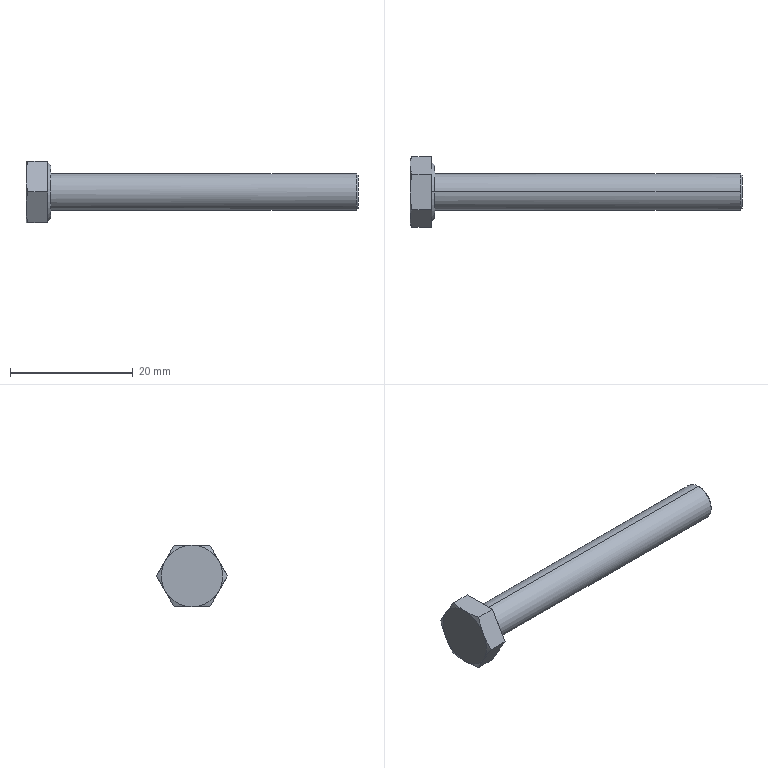Part | STEP file | hex head bolts-full thread grade c gb_GB_FASTENER_BOLT_HHBFTC M6X50-S | 1 solid | 22 faces | box 54 x 11.547 x 10 mm | volume 1749 mm3 | cone 10 | plane 10 | cylinder 2 | commonest cylinder face diameters 6 x2
STEP:
#1=CARTESIAN_POINT('',(53.7,3.,0.));
#2=VERTEX_POINT('',#1);
#3=CARTESIAN_POINT('',(53.7,0.,-3.));
#4=VERTEX_POINT('',#3);
#5=CARTESIAN_POINT('',(53.7,0.,0.));
#6=DIRECTION('',(-1.,0.,0.));
#7=DIRECTION('',(0.,0.,1.));
#8=AXIS2_PLACEMENT_3D('',#5,#6,#7);
#9=CIRCLE('',#8,3.);
#10=EDGE_CURVE('',#2,#4,#9,.T.);
#11=ORIENTED_EDGE('',*,*,#10,.T.);
#12=CARTESIAN_POINT('',(4.,0.,-3.));
#13=VERTEX_POINT('',#12);
#14=CARTESIAN_POINT('',(54.,0.,-3.));
#15=DIRECTION('',(-1.,0.,0.));
#16=VECTOR('',#15,1000.);
#17=LINE('',#14,#16);
#18=EDGE_CURVE('',#4,#13,#17,.T.);
#19=ORIENTED_EDGE('',*,*,#18,.T.);
#20=CARTESIAN_POINT('',(4.,0.,3.));
#21=VERTEX_POINT('',#20);
#22=CARTESIAN_POINT('',(4.,0.,0.));
#23=DIRECTION('',(1.,0.,0.));
#24=DIRECTION('',(0.,0.,1.));
#25=AXIS2_PLACEMENT_3D('',#22,#23,#24);
#26=CIRCLE('',#25,3.);
#27=EDGE_CURVE('',#13,#21,#26,.T.);
#28=ORIENTED_EDGE('',*,*,#27,.T.);
#29=CARTESIAN_POINT('',(53.7,0.,3.));
#30=VERTEX_POINT('',#29);
#31=CARTESIAN_POINT('',(54.,0.,3.));
#32=DIRECTION('',(-1.,0.,0.));
#33=VECTOR('',#32,1000.);
#34=LINE('',#31,#33);
#35=EDGE_CURVE('',#30,#21,#34,.T.);
#36=ORIENTED_EDGE('',*,*,#35,.F.);
#37=CARTESIAN_POINT('',(53.7,0.,0.));
#38=DIRECTION('',(-1.,0.,0.));
#39=DIRECTION('',(0.,0.,1.));
#40=AXIS2_PLACEMENT_3D('',#37,#38,#39);
#41=CIRCLE('',#40,3.);
#42=EDGE_CURVE('',#30,#2,#41,.T.);
#43=ORIENTED_EDGE('',*,*,#42,.T.);
#44=EDGE_LOOP('',(#11,#19,#28,#36,#43));
#45=FACE_OUTER_BOUND('',#44,.T.);
#46=CARTESIAN_POINT('',(54.,0.,0.));
#47=DIRECTION('',(-1.,0.,0.));
#48=DIRECTION('',(0.,0.,1.));
#49=AXIS2_PLACEMENT_3D('',#46,#47,#48);
#50=CYLINDRICAL_SURFACE('',#49,3.);
#51=ADVANCED_FACE('',(#45),#50,.T.);
#52=CARTESIAN_POINT('',(54.,-2.7,0.));
#53=VERTEX_POINT('',#52);
#54=CARTESIAN_POINT('',(54.,2.7,0.));
#55=VERTEX_POINT('',#54);
#56=CARTESIAN_POINT('',(54.,0.,0.));
#57=DIRECTION('',(-1.,0.,0.));
#58=DIRECTION('',(0.,-1.,0.));
#59=AXIS2_PLACEMENT_3D('',#56,#57,#58);
#60=CIRCLE('',#59,2.7);
#61=EDGE_CURVE('',#53,#55,#60,.T.);
#62=ORIENTED_EDGE('',*,*,#61,.T.);
#63=CARTESIAN_POINT('',(53.7,3.,0.));
#64=DIRECTION('',(-0.7071,0.7071,0.));
#65=VECTOR('',#64,1000.);
#66=LINE('',#63,#65);
#67=EDGE_CURVE('',#55,#2,#66,.T.);
#68=ORIENTED_EDGE('',*,*,#67,.T.);
#69=ORIENTED_EDGE('',*,*,#42,.F.);
#70=CARTESIAN_POINT('',(53.7,-3.,0.));
#71=VERTEX_POINT('',#70);
#72=CARTESIAN_POINT('',(53.7,0.,0.));
#73=DIRECTION('',(-1.,0.,0.));
#74=DIRECTION('',(0.,0.,1.));
#75=AXIS2_PLACEMENT_3D('',#72,#73,#74);
#76=CIRCLE('',#75,3.);
#77=EDGE_CURVE('',#71,#30,#76,.T.);
#78=ORIENTED_EDGE('',*,*,#77,.F.);
#79=CARTESIAN_POINT('',(53.7,-3.,0.));
#80=DIRECTION('',(-0.7071,-0.7071,0.));
#81=VECTOR('',#80,1000.);
#82=LINE('',#79,#81);
#83=EDGE_CURVE('',#53,#71,#82,.T.);
#84=ORIENTED_EDGE('',*,*,#83,.F.);
#85=EDGE_LOOP('',(#62,#68,#69,#78,#84));
#86=FACE_OUTER_BOUND('',#85,.T.);
#87=CARTESIAN_POINT('',(53.7,0.,0.));
#88=DIRECTION('',(-1.,0.,0.));
#89=DIRECTION('',(0.,-1.,0.));
#90=AXIS2_PLACEMENT_3D('',#87,#88,#89);
#91=CONICAL_SURFACE('',#90,3.,0.7854);
#92=ADVANCED_FACE('',(#86),#91,.T.);
#93=CARTESIAN_POINT('',(4.,0.,4.37));
#94=VERTEX_POINT('',#93);
#95=CARTESIAN_POINT('',(4.,0.,-4.37));
#96=VERTEX_POINT('',#95);
#97=CARTESIAN_POINT('',(4.,0.,0.));
#98=DIRECTION('',(-1.,0.,0.));
#99=DIRECTION('',(0.,0.,1.));
#100=AXIS2_PLACEMENT_3D('',#97,#98,#99);
#101=CIRCLE('',#100,4.37);
#102=EDGE_CURVE('',#94,#96,#101,.T.);
#103=ORIENTED_EDGE('',*,*,#102,.T.);
#104=CARTESIAN_POINT('',(3.5,0.,-4.87));
#105=VERTEX_POINT('',#104);
#106=CARTESIAN_POINT('',(3.5,0.,-4.87));
#107=DIRECTION('',(-0.7071,0.,-0.7071));
#108=VECTOR('',#107,1000.);
#109=LINE('',#106,#108);
#110=EDGE_CURVE('',#96,#105,#109,.T.);
#111=ORIENTED_EDGE('',*,*,#110,.T.);
#112=CARTESIAN_POINT('',(3.5,0.,4.87));
#113=VERTEX_POINT('',#112);
#114=CARTESIAN_POINT('',(3.5,0.,0.));
#115=DIRECTION('',(1.,0.,0.));
#116=DIRECTION('',(0.,0.,1.));
#117=AXIS2_PLACEMENT_3D('',#114,#115,#116);
#118=CIRCLE('',#117,4.87);
#119=EDGE_CURVE('',#105,#113,#118,.T.);
#120=ORIENTED_EDGE('',*,*,#119,.T.);
#121=CARTESIAN_POINT('',(3.5,0.,4.87));
#122=DIRECTION('',(-0.7071,0.,0.7071));
#123=VECTOR('',#122,1000.);
#124=LINE('',#121,#123);
#125=EDGE_CURVE('',#94,#113,#124,.T.);
#126=ORIENTED_EDGE('',*,*,#125,.F.);
#127=EDGE_LOOP('',(#103,#111,#120,#126));
#128=FACE_OUTER_BOUND('',#127,.T.);
#129=CARTESIAN_POINT('',(3.5,0.,0.));
#130=DIRECTION('',(-1.,0.,0.));
#131=DIRECTION('',(0.,0.,1.));
#132=AXIS2_PLACEMENT_3D('',#129,#130,#131);
#133=CONICAL_SURFACE('',#132,4.87,0.7854);
#134=ADVANCED_FACE('',(#128),#133,.T.);
#135=ORIENTED_EDGE('',*,*,#18,.F.);
#136=CARTESIAN_POINT('',(53.7,0.,0.));
#137=DIRECTION('',(-1.,0.,0.));
#138=DIRECTION('',(0.,0.,1.));
#139=AXIS2_PLACEMENT_3D('',#136,#137,#138);
#140=CIRCLE('',#139,3.);
#141=EDGE_CURVE('',#4,#71,#140,.T.);
#142=ORIENTED_EDGE('',*,*,#141,.T.);
#143=ORIENTED_EDGE('',*,*,#77,.T.);
#144=ORIENTED_EDGE('',*,*,#35,.T.);
#145=CARTESIAN_POINT('',(4.,0.,0.));
#146=DIRECTION('',(1.,0.,0.));
#147=DIRECTION('',(0.,0.,1.));
#148=AXIS2_PLACEMENT_3D('',#145,#146,#147);
#149=CIRCLE('',#148,3.);
#150=EDGE_CURVE('',#21,#13,#149,.T.);
#151=ORIENTED_EDGE('',*,*,#150,.T.);
#152=EDGE_LOOP('',(#135,#142,#143,#144,#151));
#153=FACE_OUTER_BOUND('',#152,.T.);
#154=CARTESIAN_POINT('',(54.,0.,0.));
#155=DIRECTION('',(-1.,0.,0.));
#156=DIRECTION('',(0.,0.,1.));
#157=AXIS2_PLACEMENT_3D('',#154,#155,#156);
#158=CYLINDRICAL_SURFACE('',#157,3.);
#159=ADVANCED_FACE('',(#153),#158,.T.);
#160=ORIENTED_EDGE('',*,*,#150,.F.);
#161=ORIENTED_EDGE('',*,*,#27,.F.);
#162=EDGE_LOOP('',(#160,#161));
#163=FACE_BOUND('',#162,.T.);
#164=ORIENTED_EDGE('',*,*,#102,.F.);
#165=CARTESIAN_POINT('',(4.,0.,0.));
#166=DIRECTION('',(-1.,0.,0.));
#167=DIRECTION('',(0.,0.,1.));
#168=AXIS2_PLACEMENT_3D('',#165,#166,#167);
#169=CIRCLE('',#168,4.37);
#170=EDGE_CURVE('',#96,#94,#169,.T.);
#171=ORIENTED_EDGE('',*,*,#170,.F.);
#172=EDGE_LOOP('',(#164,#171));
#173=FACE_OUTER_BOUND('',#172,.T.);
#174=CARTESIAN_POINT('',(4.,0.,10.));
#175=DIRECTION('',(-1.,0.,0.));
#176=DIRECTION('',(0.,0.,1.));
#177=AXIS2_PLACEMENT_3D('',#174,#175,#176);
#178=PLANE('',#177);
#179=ADVANCED_FACE('',(#163,#173),#178,.F.);
#180=ORIENTED_EDGE('',*,*,#67,.F.);
#181=CARTESIAN_POINT('',(54.,0.,0.));
#182=DIRECTION('',(-1.,0.,0.));
#183=DIRECTION('',(0.,-1.,0.));
#184=AXIS2_PLACEMENT_3D('',#181,#182,#183);
#185=CIRCLE('',#184,2.7);
#186=EDGE_CURVE('',#55,#53,#185,.T.);
#187=ORIENTED_EDGE('',*,*,#186,.T.);
#188=ORIENTED_EDGE('',*,*,#83,.T.);
#189=ORIENTED_EDGE('',*,*,#141,.F.);
#190=ORIENTED_EDGE('',*,*,#10,.F.);
#191=EDGE_LOOP('',(#180,#187,#188,#189,#190));
#192=FACE_OUTER_BOUND('',#191,.T.);
#193=CARTESIAN_POINT('',(53.7,0.,0.));
#194=DIRECTION('',(-1.,0.,0.));
#195=DIRECTION('',(0.,-1.,0.));
#196=AXIS2_PLACEMENT_3D('',#193,#194,#195);
#197=CONICAL_SURFACE('',#196,3.,0.7854);
#198=ADVANCED_FACE('',(#192),#197,.T.);
#199=ORIENTED_EDGE('',*,*,#110,.F.);
#200=ORIENTED_EDGE('',*,*,#170,.T.);
#201=ORIENTED_EDGE('',*,*,#125,.T.);
#202=CARTESIAN_POINT('',(3.5,0.,0.));
#203=DIRECTION('',(1.,0.,0.));
#204=DIRECTION('',(0.,0.,1.));
#205=AXIS2_PLACEMENT_3D('',#202,#203,#204);
#206=CIRCLE('',#205,4.87);
#207=EDGE_CURVE('',#113,#105,#206,.T.);
#208=ORIENTED_EDGE('',*,*,#207,.T.);
#209=EDGE_LOOP('',(#199,#200,#201,#208));
#210=FACE_OUTER_BOUND('',#209,.T.);
#211=CARTESIAN_POINT('',(3.5,0.,0.));
#212=DIRECTION('',(-1.,0.,0.));
#213=DIRECTION('',(0.,0.,1.));
#214=AXIS2_PLACEMENT_3D('',#211,#212,#213);
#215=CONICAL_SURFACE('',#214,4.87,0.7854);
#216=ADVANCED_FACE('',(#210),#215,.T.);
#217=ORIENTED_EDGE('',*,*,#61,.F.);
#218=ORIENTED_EDGE('',*,*,#186,.F.);
#219=EDGE_LOOP('',(#217,#218));
#220=FACE_OUTER_BOUND('',#219,.T.);
#221=CARTESIAN_POINT('',(54.,0.,0.));
#222=DIRECTION('',(1.,0.,0.));
#223=DIRECTION('',(0.,0.,-1.));
#224=AXIS2_PLACEMENT_3D('',#221,#222,#223);
#225=PLANE('',#224);
#226=ADVANCED_FACE('',(#220),#225,.T.);
#227=CARTESIAN_POINT('',(3.5,5.774,0.));
#228=VERTEX_POINT('',#227);
#229=CARTESIAN_POINT('',(3.5,2.887,5.));
#230=VERTEX_POINT('',#229);
#231=CARTESIAN_POINT('',(3.5,5.774,0.));
#232=DIRECTION('',(0.,-0.5,0.866));
#233=VECTOR('',#232,1000.);
#234=LINE('',#231,#233);
#235=EDGE_CURVE('',#228,#230,#234,.T.);
#236=ORIENTED_EDGE('',*,*,#235,.T.);
#237=CARTESIAN_POINT('',(3.5,-2.887,5.));
#238=VERTEX_POINT('',#237);
#239=CARTESIAN_POINT('',(3.5,4.87,5.));
#240=DIRECTION('',(0.,-1.,0.));
#241=VECTOR('',#240,1000.);
#242=LINE('',#239,#241);
#243=EDGE_CURVE('',#230,#238,#242,.T.);
#244=ORIENTED_EDGE('',*,*,#243,.T.);
#245=CARTESIAN_POINT('',(3.5,-5.774,0.));
#246=VERTEX_POINT('',#245);
#247=CARTESIAN_POINT('',(3.5,-2.887,5.));
#248=DIRECTION('',(0.,-0.5,-0.866));
#249=VECTOR('',#248,1000.);
#250=LINE('',#247,#249);
#251=EDGE_CURVE('',#238,#246,#250,.T.);
#252=ORIENTED_EDGE('',*,*,#251,.T.);
#253=CARTESIAN_POINT('',(3.5,-2.887,-5.));
#254=VERTEX_POINT('',#253);
#255=CARTESIAN_POINT('',(3.5,-5.774,0.));
#256=DIRECTION('',(0.,0.5,-0.866));
#257=VECTOR('',#256,1000.);
#258=LINE('',#255,#257);
#259=EDGE_CURVE('',#246,#254,#258,.T.);
#260=ORIENTED_EDGE('',*,*,#259,.T.);
#261=CARTESIAN_POINT('',(3.5,2.887,-5.));
#262=VERTEX_POINT('',#261);
#263=CARTESIAN_POINT('',(3.5,4.87,-5.));
#264=DIRECTION('',(0.,1.,0.));
#265=VECTOR('',#264,1000.);
#266=LINE('',#263,#265);
#267=EDGE_CURVE('',#254,#262,#266,.T.);
#268=ORIENTED_EDGE('',*,*,#267,.T.);
#269=CARTESIAN_POINT('',(3.5,2.887,-5.));
#270=DIRECTION('',(0.,0.5,0.866));
#271=VECTOR('',#270,1000.);
#272=LINE('',#269,#271);
#273=EDGE_CURVE('',#262,#228,#272,.T.);
#274=ORIENTED_EDGE('',*,*,#273,.T.);
#275=EDGE_LOOP('',(#236,#244,#252,#260,#268,#274));
#276=FACE_OUTER_BOUND('',#275,.T.);
#277=ORIENTED_EDGE('',*,*,#207,.F.);
#278=ORIENTED_EDGE('',*,*,#119,.F.);
#279=EDGE_LOOP('',(#277,#278));
#280=FACE_BOUND('',#279,.T.);
#281=CARTESIAN_POINT('',(3.5,4.87,0.));
#282=DIRECTION('',(1.,0.,0.));
#283=DIRECTION('',(0.,0.,-1.));
#284=AXIS2_PLACEMENT_3D('',#281,#282,#283);
#285=PLANE('',#284);
#286=ADVANCED_FACE('',(#276,#280),#285,.T.);
#287=CARTESIAN_POINT('',(0.2815,-2.887,5.));
#288=VERTEX_POINT('',#287);
#289=CARTESIAN_POINT('',(4.,-2.887,5.));
#290=DIRECTION('',(-1.,0.,0.));
#291=VECTOR('',#290,1000.);
#292=LINE('',#289,#291);
#293=EDGE_CURVE('',#238,#288,#292,.T.);
#294=ORIENTED_EDGE('',*,*,#293,.F.);
#295=ORIENTED_EDGE('',*,*,#243,.F.);
#296=CARTESIAN_POINT('',(0.2815,2.887,5.));
#297=VERTEX_POINT('',#296);
#298=CARTESIAN_POINT('',(4.,2.887,5.));
#299=DIRECTION('',(1.,0.,0.));
#300=VECTOR('',#299,1000.);
#301=LINE('',#298,#300);
#302=EDGE_CURVE('',#297,#230,#301,.T.);
#303=ORIENTED_EDGE('',*,*,#302,.F.);
#304=CARTESIAN_POINT('',(0.,0.,5.));
#305=VERTEX_POINT('',#304);
#306=CARTESIAN_POINT('',(0.,0.,5.));
#307=CARTESIAN_POINT('',(0.,0.9714,5.));
#308=CARTESIAN_POINT('',(0.1078,1.932,5.));
#309=CARTESIAN_POINT('',(0.2815,2.887,5.));
#310=B_SPLINE_CURVE_WITH_KNOTS('',3,(#306,#307,#308,#309),.UNSPECIFIED.,.F.,.F.,(4,4),(0.,0.0029),.UNSPECIFIED.);
#311=EDGE_CURVE('',#305,#297,#310,.T.);
#312=ORIENTED_EDGE('',*,*,#311,.F.);
#313=CARTESIAN_POINT('',(0.2815,-2.887,5.));
#314=CARTESIAN_POINT('',(0.1078,-1.932,5.));
#315=CARTESIAN_POINT('',(0.,-0.9714,5.));
#316=CARTESIAN_POINT('',(0.,0.,5.));
#317=B_SPLINE_CURVE_WITH_KNOTS('',3,(#313,#314,#315,#316),.UNSPECIFIED.,.F.,.F.,(4,4),(0.,0.0029),.UNSPECIFIED.);
#318=EDGE_CURVE('',#288,#305,#317,.T.);
#319=ORIENTED_EDGE('',*,*,#318,.F.);
#320=EDGE_LOOP('',(#294,#295,#303,#312,#319));
#321=FACE_OUTER_BOUND('',#320,.T.);
#322=CARTESIAN_POINT('',(4.,2.887,5.));
#323=DIRECTION('',(0.,0.,-1.));
#324=DIRECTION('',(0.,1.,0.));
#325=AXIS2_PLACEMENT_3D('',#322,#323,#324);
#326=PLANE('',#325);
#327=ADVANCED_FACE('',(#321),#326,.F.);
#328=ORIENTED_EDGE('',*,*,#302,.T.);
#329=ORIENTED_EDGE('',*,*,#235,.F.);
#330=CARTESIAN_POINT('',(0.2815,5.774,0.));
#331=VERTEX_POINT('',#330);
#332=CARTESIAN_POINT('',(4.,5.774,0.));
#333=DIRECTION('',(1.,0.,0.));
#334=VECTOR('',#333,1000.);
#335=LINE('',#332,#334);
#336=EDGE_CURVE('',#331,#228,#335,.T.);
#337=ORIENTED_EDGE('',*,*,#336,.F.);
#338=CARTESIAN_POINT('',(0.,4.33,2.5));
#339=VERTEX_POINT('',#338);
#340=CARTESIAN_POINT('',(0.,4.33,2.5));
#341=CARTESIAN_POINT('',(0.,4.816,1.659));
#342=CARTESIAN_POINT('',(0.1078,5.296,0.8266));
#343=CARTESIAN_POINT('',(0.2815,5.774,0.));
#344=B_SPLINE_CURVE_WITH_KNOTS('',3,(#340,#341,#342,#343),.UNSPECIFIED.,.F.,.F.,(4,4),(0.,0.0029),.UNSPECIFIED.);
#345=EDGE_CURVE('',#339,#331,#344,.T.);
#346=ORIENTED_EDGE('',*,*,#345,.F.);
#347=CARTESIAN_POINT('',(0.2815,2.887,5.));
#348=CARTESIAN_POINT('',(0.1078,3.364,4.173));
#349=CARTESIAN_POINT('',(0.,3.844,3.341));
#350=CARTESIAN_POINT('',(0.,4.33,2.5));
#351=B_SPLINE_CURVE_WITH_KNOTS('',3,(#347,#348,#349,#350),.UNSPECIFIED.,.F.,.F.,(4,4),(0.,0.0029),.UNSPECIFIED.);
#352=EDGE_CURVE('',#297,#339,#351,.T.);
#353=ORIENTED_EDGE('',*,*,#352,.F.);
#354=EDGE_LOOP('',(#328,#329,#337,#346,#353));
#355=FACE_OUTER_BOUND('',#354,.T.);
#356=CARTESIAN_POINT('',(4.,5.774,0.));
#357=DIRECTION('',(0.,-0.866,-0.5));
#358=DIRECTION('',(0.,0.5,-0.866));
#359=AXIS2_PLACEMENT_3D('',#356,#357,#358);
#360=PLANE('',#359);
#361=ADVANCED_FACE('',(#355),#360,.F.);
#362=ORIENTED_EDGE('',*,*,#336,.T.);
#363=ORIENTED_EDGE('',*,*,#273,.F.);
#364=CARTESIAN_POINT('',(0.2815,2.887,-5.));
#365=VERTEX_POINT('',#364);
#366=CARTESIAN_POINT('',(4.,2.887,-5.));
#367=DIRECTION('',(1.,0.,0.));
#368=VECTOR('',#367,1000.);
#369=LINE('',#366,#368);
#370=EDGE_CURVE('',#365,#262,#369,.T.);
#371=ORIENTED_EDGE('',*,*,#370,.F.);
#372=CARTESIAN_POINT('',(0.,4.33,-2.5));
#373=VERTEX_POINT('',#372);
#374=CARTESIAN_POINT('',(0.,4.33,-2.5));
#375=CARTESIAN_POINT('',(0.,3.844,-3.341));
#376=CARTESIAN_POINT('',(0.1078,3.364,-4.173));
#377=CARTESIAN_POINT('',(0.2815,2.887,-5.));
#378=B_SPLINE_CURVE_WITH_KNOTS('',3,(#374,#375,#376,#377),.UNSPECIFIED.,.F.,.F.,(4,4),(0.,0.0029),.UNSPECIFIED.);
#379=EDGE_CURVE('',#373,#365,#378,.T.);
#380=ORIENTED_EDGE('',*,*,#379,.F.);
#381=CARTESIAN_POINT('',(0.2815,5.774,0.));
#382=CARTESIAN_POINT('',(0.1078,5.296,-0.8266));
#383=CARTESIAN_POINT('',(0.,4.816,-1.659));
#384=CARTESIAN_POINT('',(0.,4.33,-2.5));
#385=B_SPLINE_CURVE_WITH_KNOTS('',3,(#381,#382,#383,#384),.UNSPECIFIED.,.F.,.F.,(4,4),(0.,0.0029),.UNSPECIFIED.);
#386=EDGE_CURVE('',#331,#373,#385,.T.);
#387=ORIENTED_EDGE('',*,*,#386,.F.);
#388=EDGE_LOOP('',(#362,#363,#371,#380,#387));
#389=FACE_OUTER_BOUND('',#388,.T.);
#390=CARTESIAN_POINT('',(4.,2.887,-5.));
#391=DIRECTION('',(0.,-0.866,0.5));
#392=DIRECTION('',(0.,-0.5,-0.866));
#393=AXIS2_PLACEMENT_3D('',#390,#391,#392);
#394=PLANE('',#393);
#395=ADVANCED_FACE('',(#389),#394,.F.);
#396=ORIENTED_EDGE('',*,*,#370,.T.);
#397=ORIENTED_EDGE('',*,*,#267,.F.);
#398=CARTESIAN_POINT('',(0.2815,-2.887,-5.));
#399=VERTEX_POINT('',#398);
#400=CARTESIAN_POINT('',(4.,-2.887,-5.));
#401=DIRECTION('',(1.,0.,0.));
#402=VECTOR('',#401,1000.);
#403=LINE('',#400,#402);
#404=EDGE_CURVE('',#399,#254,#403,.T.);
#405=ORIENTED_EDGE('',*,*,#404,.F.);
#406=CARTESIAN_POINT('',(0.,0.,-5.));
#407=VERTEX_POINT('',#406);
#408=CARTESIAN_POINT('',(0.,0.,-5.));
#409=CARTESIAN_POINT('',(0.,-0.9714,-5.));
#410=CARTESIAN_POINT('',(0.1078,-1.932,-5.));
#411=CARTESIAN_POINT('',(0.2815,-2.887,-5.));
#412=B_SPLINE_CURVE_WITH_KNOTS('',3,(#408,#409,#410,#411),.UNSPECIFIED.,.F.,.F.,(4,4),(0.,0.0029),.UNSPECIFIED.);
#413=EDGE_CURVE('',#407,#399,#412,.T.);
#414=ORIENTED_EDGE('',*,*,#413,.F.);
#415=CARTESIAN_POINT('',(0.2815,2.887,-5.));
#416=CARTESIAN_POINT('',(0.1078,1.932,-5.));
#417=CARTESIAN_POINT('',(0.,0.9714,-5.));
#418=CARTESIAN_POINT('',(0.,0.,-5.));
#419=B_SPLINE_CURVE_WITH_KNOTS('',3,(#415,#416,#417,#418),.UNSPECIFIED.,.F.,.F.,(4,4),(0.,0.0029),.UNSPECIFIED.);
#420=EDGE_CURVE('',#365,#407,#419,.T.);
#421=ORIENTED_EDGE('',*,*,#420,.F.);
#422=EDGE_LOOP('',(#396,#397,#405,#414,#421));
#423=FACE_OUTER_BOUND('',#422,.T.);
#424=CARTESIAN_POINT('',(4.,-2.887,-5.));
#425=DIRECTION('',(0.,0.,1.));
#426=DIRECTION('',(1.,0.,0.));
#427=AXIS2_PLACEMENT_3D('',#424,#425,#426);
#428=PLANE('',#427);
#429=ADVANCED_FACE('',(#423),#428,.F.);
#430=ORIENTED_EDGE('',*,*,#404,.T.);
#431=ORIENTED_EDGE('',*,*,#259,.F.);
#432=CARTESIAN_POINT('',(0.2815,-5.774,0.));
#433=VERTEX_POINT('',#432);
#434=CARTESIAN_POINT('',(4.,-5.774,0.));
#435=DIRECTION('',(1.,0.,0.));
#436=VECTOR('',#435,1000.);
#437=LINE('',#434,#436);
#438=EDGE_CURVE('',#433,#246,#437,.T.);
#439=ORIENTED_EDGE('',*,*,#438,.F.);
#440=CARTESIAN_POINT('',(0.,-4.33,-2.5));
#441=VERTEX_POINT('',#440);
#442=CARTESIAN_POINT('',(0.,-4.33,-2.5));
#443=CARTESIAN_POINT('',(0.,-4.816,-1.659));
#444=CARTESIAN_POINT('',(0.1078,-5.296,-0.8266));
#445=CARTESIAN_POINT('',(0.2815,-5.774,0.));
#446=B_SPLINE_CURVE_WITH_KNOTS('',3,(#442,#443,#444,#445),.UNSPECIFIED.,.F.,.F.,(4,4),(0.,0.0029),.UNSPECIFIED.);
#447=EDGE_CURVE('',#441,#433,#446,.T.);
#448=ORIENTED_EDGE('',*,*,#447,.F.);
#449=CARTESIAN_POINT('',(0.2815,-2.887,-5.));
#450=CARTESIAN_POINT('',(0.1078,-3.364,-4.173));
#451=CARTESIAN_POINT('',(0.,-3.844,-3.341));
#452=CARTESIAN_POINT('',(0.,-4.33,-2.5));
#453=B_SPLINE_CURVE_WITH_KNOTS('',3,(#449,#450,#451,#452),.UNSPECIFIED.,.F.,.F.,(4,4),(0.,0.0029),.UNSPECIFIED.);
#454=EDGE_CURVE('',#399,#441,#453,.T.);
#455=ORIENTED_EDGE('',*,*,#454,.F.);
#456=EDGE_LOOP('',(#430,#431,#439,#448,#455));
#457=FACE_OUTER_BOUND('',#456,.T.);
#458=CARTESIAN_POINT('',(4.,-5.774,0.));
#459=DIRECTION('',(0.,0.866,0.5));
#460=DIRECTION('',(0.,-0.5,0.866));
#461=AXIS2_PLACEMENT_3D('',#458,#459,#460);
#462=PLANE('',#461);
#463=ADVANCED_FACE('',(#457),#462,.F.);
#464=ORIENTED_EDGE('',*,*,#438,.T.);
#465=ORIENTED_EDGE('',*,*,#251,.F.);
#466=ORIENTED_EDGE('',*,*,#293,.T.);
#467=CARTESIAN_POINT('',(0.,-4.33,2.5));
#468=VERTEX_POINT('',#467);
#469=CARTESIAN_POINT('',(0.,-4.33,2.5));
#470=CARTESIAN_POINT('',(0.,-3.844,3.341));
#471=CARTESIAN_POINT('',(0.1078,-3.364,4.173));
#472=CARTESIAN_POINT('',(0.2815,-2.887,5.));
#473=B_SPLINE_CURVE_WITH_KNOTS('',3,(#469,#470,#471,#472),.UNSPECIFIED.,.F.,.F.,(4,4),(0.,0.0029),.UNSPECIFIED.);
#474=EDGE_CURVE('',#468,#288,#473,.T.);
#475=ORIENTED_EDGE('',*,*,#474,.F.);
#476=CARTESIAN_POINT('',(0.2815,-5.774,0.));
#477=CARTESIAN_POINT('',(0.1078,-5.296,0.8266));
#478=CARTESIAN_POINT('',(0.,-4.816,1.659));
#479=CARTESIAN_POINT('',(0.,-4.33,2.5));
#480=B_SPLINE_CURVE_WITH_KNOTS('',3,(#476,#477,#478,#479),.UNSPECIFIED.,.F.,.F.,(4,4),(0.,0.0029),.UNSPECIFIED.);
#481=EDGE_CURVE('',#433,#468,#480,.T.);
#482=ORIENTED_EDGE('',*,*,#481,.F.);
#483=EDGE_LOOP('',(#464,#465,#466,#475,#482));
#484=FACE_OUTER_BOUND('',#483,.T.);
#485=CARTESIAN_POINT('',(4.,-2.887,5.));
#486=DIRECTION('',(0.,0.866,-0.5));
#487=DIRECTION('',(0.,0.5,0.866));
#488=AXIS2_PLACEMENT_3D('',#485,#486,#487);
#489=PLANE('',#488);
#490=ADVANCED_FACE('',(#484),#489,.F.);
#491=ORIENTED_EDGE('',*,*,#318,.T.);
#492=CARTESIAN_POINT('',(0.,0.,0.));
#493=DIRECTION('',(1.,0.,0.));
#494=DIRECTION('',(0.,0.,-1.));
#495=AXIS2_PLACEMENT_3D('',#492,#493,#494);
#496=CIRCLE('',#495,5.);
#497=EDGE_CURVE('',#305,#468,#496,.T.);
#498=ORIENTED_EDGE('',*,*,#497,.T.);
#499=ORIENTED_EDGE('',*,*,#474,.T.);
#500=EDGE_LOOP('',(#491,#498,#499));
#501=FACE_OUTER_BOUND('',#500,.T.);
#502=CARTESIAN_POINT('',(0.2832,0.,0.));
#503=DIRECTION('',(1.,0.,0.));
#504=DIRECTION('',(0.,0.,-1.));
#505=AXIS2_PLACEMENT_3D('',#502,#503,#504);
#506=CONICAL_SURFACE('',#505,5.778,1.222);
#507=ADVANCED_FACE('',(#501),#506,.T.);
#508=CARTESIAN_POINT('',(0.,0.,0.));
#509=DIRECTION('',(1.,0.,0.));
#510=DIRECTION('',(0.,0.,-1.));
#511=AXIS2_PLACEMENT_3D('',#508,#509,#510);
#512=CIRCLE('',#511,5.);
#513=EDGE_CURVE('',#339,#305,#512,.T.);
#514=ORIENTED_EDGE('',*,*,#513,.T.);
#515=ORIENTED_EDGE('',*,*,#311,.T.);
#516=ORIENTED_EDGE('',*,*,#352,.T.);
#517=EDGE_LOOP('',(#514,#515,#516));
#518=FACE_OUTER_BOUND('',#517,.T.);
#519=CARTESIAN_POINT('',(0.2832,0.,0.));
#520=DIRECTION('',(1.,0.,0.));
#521=DIRECTION('',(0.,0.,-1.));
#522=AXIS2_PLACEMENT_3D('',#519,#520,#521);
#523=CONICAL_SURFACE('',#522,5.778,1.222);
#524=ADVANCED_FACE('',(#518),#523,.T.);
#525=CARTESIAN_POINT('',(0.,0.,0.));
#526=DIRECTION('',(1.,0.,0.));
#527=DIRECTION('',(0.,0.,-1.));
#528=AXIS2_PLACEMENT_3D('',#525,#526,#527);
#529=CIRCLE('',#528,5.);
#530=EDGE_CURVE('',#373,#339,#529,.T.);
#531=ORIENTED_EDGE('',*,*,#530,.T.);
#532=ORIENTED_EDGE('',*,*,#345,.T.);
#533=ORIENTED_EDGE('',*,*,#386,.T.);
#534=EDGE_LOOP('',(#531,#532,#533));
#535=FACE_OUTER_BOUND('',#534,.T.);
#536=CARTESIAN_POINT('',(0.2832,0.,0.));
#537=DIRECTION('',(1.,0.,0.));
#538=DIRECTION('',(0.,0.,-1.));
#539=AXIS2_PLACEMENT_3D('',#536,#537,#538);
#540=CONICAL_SURFACE('',#539,5.778,1.222);
#541=ADVANCED_FACE('',(#535),#540,.T.);
#542=CARTESIAN_POINT('',(0.,0.,0.));
#543=DIRECTION('',(1.,0.,0.));
#544=DIRECTION('',(0.,0.,-1.));
#545=AXIS2_PLACEMENT_3D('',#542,#543,#544);
#546=CIRCLE('',#545,5.);
#547=EDGE_CURVE('',#407,#373,#546,.T.);
#548=ORIENTED_EDGE('',*,*,#547,.T.);
#549=ORIENTED_EDGE('',*,*,#379,.T.);
#550=ORIENTED_EDGE('',*,*,#420,.T.);
#551=EDGE_LOOP('',(#548,#549,#550));
#552=FACE_OUTER_BOUND('',#551,.T.);
#553=CARTESIAN_POINT('',(0.2832,0.,0.));
#554=DIRECTION('',(1.,0.,0.));
#555=DIRECTION('',(0.,0.,-1.));
#556=AXIS2_PLACEMENT_3D('',#553,#554,#555);
#557=CONICAL_SURFACE('',#556,5.778,1.222);
#558=ADVANCED_FACE('',(#552),#557,.T.);
#559=ORIENTED_EDGE('',*,*,#454,.T.);
#560=CARTESIAN_POINT('',(0.,0.,0.));
#561=DIRECTION('',(1.,0.,0.));
#562=DIRECTION('',(0.,0.,-1.));
#563=AXIS2_PLACEMENT_3D('',#560,#561,#562);
#564=CIRCLE('',#563,5.);
#565=EDGE_CURVE('',#441,#407,#564,.T.);
#566=ORIENTED_EDGE('',*,*,#565,.T.);
#567=ORIENTED_EDGE('',*,*,#413,.T.);
#568=EDGE_LOOP('',(#559,#566,#567));
#569=FACE_OUTER_BOUND('',#568,.T.);
#570=CARTESIAN_POINT('',(0.2832,0.,0.));
#571=DIRECTION('',(1.,0.,0.));
#572=DIRECTION('',(0.,0.,-1.));
#573=AXIS2_PLACEMENT_3D('',#570,#571,#572);
#574=CONICAL_SURFACE('',#573,5.778,1.222);
#575=ADVANCED_FACE('',(#569),#574,.T.);
#576=ORIENTED_EDGE('',*,*,#481,.T.);
#577=CARTESIAN_POINT('',(0.,0.,0.));
#578=DIRECTION('',(1.,0.,0.));
#579=DIRECTION('',(0.,0.,-1.));
#580=AXIS2_PLACEMENT_3D('',#577,#578,#579);
#581=CIRCLE('',#580,5.);
#582=EDGE_CURVE('',#468,#441,#581,.T.);
#583=ORIENTED_EDGE('',*,*,#582,.T.);
#584=ORIENTED_EDGE('',*,*,#447,.T.);
#585=EDGE_LOOP('',(#576,#583,#584));
#586=FACE_OUTER_BOUND('',#585,.T.);
#587=CARTESIAN_POINT('',(0.2832,0.,0.));
#588=DIRECTION('',(1.,0.,0.));
#589=DIRECTION('',(0.,0.,-1.));
#590=AXIS2_PLACEMENT_3D('',#587,#588,#589);
#591=CONICAL_SURFACE('',#590,5.778,1.222);
#592=ADVANCED_FACE('',(#586),#591,.T.);
#593=ORIENTED_EDGE('',*,*,#565,.F.);
#594=ORIENTED_EDGE('',*,*,#582,.F.);
#595=ORIENTED_EDGE('',*,*,#497,.F.);
#596=ORIENTED_EDGE('',*,*,#513,.F.);
#597=ORIENTED_EDGE('',*,*,#530,.F.);
#598=ORIENTED_EDGE('',*,*,#547,.F.);
#599=EDGE_LOOP('',(#593,#594,#595,#596,#597,#598));
#600=FACE_OUTER_BOUND('',#599,.T.);
#601=CARTESIAN_POINT('',(0.,0.,10.));
#602=DIRECTION('',(-1.,0.,0.));
#603=DIRECTION('',(0.,0.,1.));
#604=AXIS2_PLACEMENT_3D('',#601,#602,#603);
#605=PLANE('',#604);
#606=ADVANCED_FACE('',(#600),#605,.T.);
#607=CLOSED_SHELL('',(#51,#92,#134,#159,#179,#198,#216,#226,#286,#327,#361,#395,#429,#463,#490,#507,#524,#541,#558,#575,#592,#606));
#608=MANIFOLD_SOLID_BREP('',#607);
#609=CARTESIAN_POINT('',(0.,0.,0.));
#610=DIRECTION('',(0.,0.,1.));
#611=DIRECTION('',(1.,0.,0.));
#612=AXIS2_PLACEMENT_3D('',#609,#610,#611);
#613=(LENGTH_UNIT()NAMED_UNIT(*)SI_UNIT(.MILLI.,.METRE.));
#614=UNCERTAINTY_MEASURE_WITH_UNIT(LENGTH_MEASURE(0.00001),#613,'','');
#615=(NAMED_UNIT(*)PLANE_ANGLE_UNIT()SI_UNIT($,.RADIAN.));
#616=(NAMED_UNIT(*)SI_UNIT($,.STERADIAN.)SOLID_ANGLE_UNIT());
#617=(GEOMETRIC_REPRESENTATION_CONTEXT(3)GLOBAL_UNCERTAINTY_ASSIGNED_CONTEXT((#614))GLOBAL_UNIT_ASSIGNED_CONTEXT((#613,#615,#616))REPRESENTATION_CONTEXT('',''));
#618=ADVANCED_BREP_SHAPE_REPRESENTATION('',(#608,#612),#617);